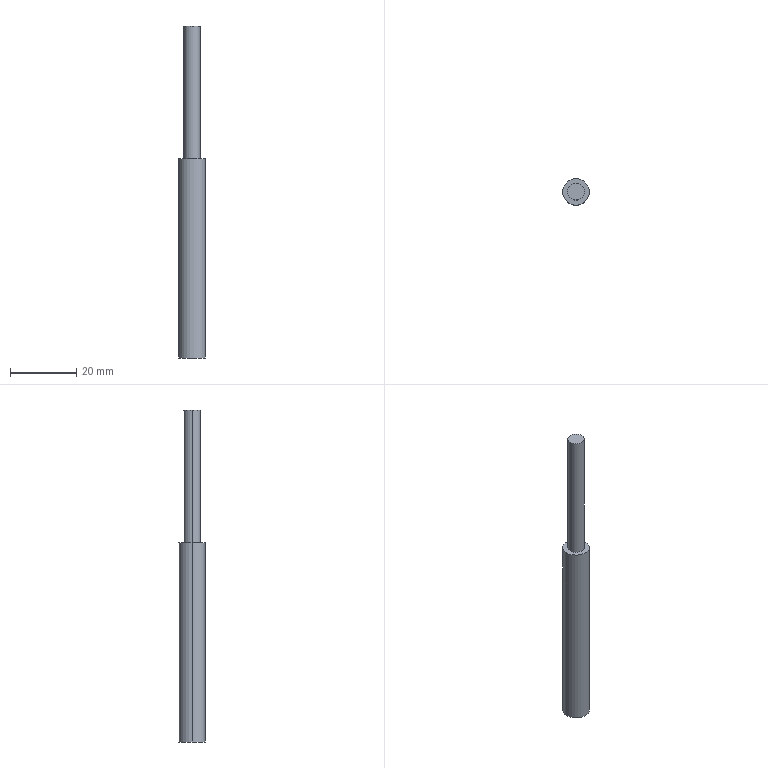Part | SolidWorks | features Extrusion 1, ICE 1 | 1 solid | 7 faces | box 8 x 8 x 100 mm | volume 3801 mm3 | cylinder 4 | plane 3 | commonest cylinder face diameters 5 x2 8 x2
STEP:
#1=CARTESIAN_POINT('',(2.5,0.,60.));
#2=VERTEX_POINT('',#1);
#3=CARTESIAN_POINT('',(-2.5,0.,60.));
#4=VERTEX_POINT('',#3);
#5=CARTESIAN_POINT('',(0.,0.,60.));
#6=DIRECTION('',(0.,0.,1.));
#7=DIRECTION('',(1.,0.,0.));
#8=AXIS2_PLACEMENT_3D('',#5,#6,#7);
#9=CIRCLE('',#8,2.5);
#10=EDGE_CURVE('',#2,#4,#9,.T.);
#11=ORIENTED_EDGE('',*,*,#10,.T.);
#12=CARTESIAN_POINT('',(-2.5,0.,100.));
#13=VERTEX_POINT('',#12);
#14=CARTESIAN_POINT('',(-2.5,0.,60.));
#15=DIRECTION('',(0.,0.,1.));
#16=VECTOR('',#15,1000.);
#17=LINE('',#14,#16);
#18=EDGE_CURVE('',#4,#13,#17,.T.);
#19=ORIENTED_EDGE('',*,*,#18,.T.);
#20=CARTESIAN_POINT('',(2.5,0.,100.));
#21=VERTEX_POINT('',#20);
#22=CARTESIAN_POINT('',(0.,0.,100.));
#23=DIRECTION('',(0.,0.,1.));
#24=DIRECTION('',(1.,0.,0.));
#25=AXIS2_PLACEMENT_3D('',#22,#23,#24);
#26=CIRCLE('',#25,2.5);
#27=EDGE_CURVE('',#21,#13,#26,.T.);
#28=ORIENTED_EDGE('',*,*,#27,.F.);
#29=CARTESIAN_POINT('',(2.5,0.,60.));
#30=DIRECTION('',(0.,0.,1.));
#31=VECTOR('',#30,1000.);
#32=LINE('',#29,#31);
#33=EDGE_CURVE('',#2,#21,#32,.T.);
#34=ORIENTED_EDGE('',*,*,#33,.F.);
#35=EDGE_LOOP('',(#11,#19,#28,#34));
#36=FACE_OUTER_BOUND('',#35,.T.);
#37=CARTESIAN_POINT('',(0.,0.,60.));
#38=DIRECTION('',(0.,0.,1.));
#39=DIRECTION('',(1.,0.,0.));
#40=AXIS2_PLACEMENT_3D('',#37,#38,#39);
#41=CYLINDRICAL_SURFACE('',#40,2.5);
#42=ADVANCED_FACE('',(#36),#41,.T.);
#43=CARTESIAN_POINT('',(4.,0.,60.));
#44=VERTEX_POINT('',#43);
#45=CARTESIAN_POINT('',(-4.,0.,60.));
#46=VERTEX_POINT('',#45);
#47=CARTESIAN_POINT('',(0.,0.,60.));
#48=DIRECTION('',(0.,0.,1.));
#49=DIRECTION('',(1.,0.,0.));
#50=AXIS2_PLACEMENT_3D('',#47,#48,#49);
#51=CIRCLE('',#50,4.);
#52=EDGE_CURVE('',#44,#46,#51,.T.);
#53=ORIENTED_EDGE('',*,*,#52,.F.);
#54=CARTESIAN_POINT('',(4.,0.,0.));
#55=VERTEX_POINT('',#54);
#56=CARTESIAN_POINT('',(4.,0.,100.));
#57=DIRECTION('',(0.,0.,-1.));
#58=VECTOR('',#57,1000.);
#59=LINE('',#56,#58);
#60=EDGE_CURVE('',#44,#55,#59,.T.);
#61=ORIENTED_EDGE('',*,*,#60,.T.);
#62=CARTESIAN_POINT('',(-4.,0.,0.));
#63=VERTEX_POINT('',#62);
#64=CARTESIAN_POINT('',(0.,0.,0.));
#65=DIRECTION('',(0.,0.,1.));
#66=DIRECTION('',(1.,0.,0.));
#67=AXIS2_PLACEMENT_3D('',#64,#65,#66);
#68=CIRCLE('',#67,4.);
#69=EDGE_CURVE('',#55,#63,#68,.T.);
#70=ORIENTED_EDGE('',*,*,#69,.T.);
#71=CARTESIAN_POINT('',(-4.,0.,100.));
#72=DIRECTION('',(0.,0.,-1.));
#73=VECTOR('',#72,1000.);
#74=LINE('',#71,#73);
#75=EDGE_CURVE('',#46,#63,#74,.T.);
#76=ORIENTED_EDGE('',*,*,#75,.F.);
#77=EDGE_LOOP('',(#53,#61,#70,#76));
#78=FACE_OUTER_BOUND('',#77,.T.);
#79=CARTESIAN_POINT('',(0.,0.,100.));
#80=DIRECTION('',(0.,0.,-1.));
#81=DIRECTION('',(-1.,0.,0.));
#82=AXIS2_PLACEMENT_3D('',#79,#80,#81);
#83=CYLINDRICAL_SURFACE('',#82,4.);
#84=ADVANCED_FACE('',(#78),#83,.T.);
#85=ORIENTED_EDGE('',*,*,#60,.F.);
#86=CARTESIAN_POINT('',(0.,0.,60.));
#87=DIRECTION('',(0.,0.,1.));
#88=DIRECTION('',(1.,0.,0.));
#89=AXIS2_PLACEMENT_3D('',#86,#87,#88);
#90=CIRCLE('',#89,4.);
#91=EDGE_CURVE('',#46,#44,#90,.T.);
#92=ORIENTED_EDGE('',*,*,#91,.F.);
#93=ORIENTED_EDGE('',*,*,#75,.T.);
#94=CARTESIAN_POINT('',(0.,0.,0.));
#95=DIRECTION('',(0.,0.,1.));
#96=DIRECTION('',(1.,0.,0.));
#97=AXIS2_PLACEMENT_3D('',#94,#95,#96);
#98=CIRCLE('',#97,4.);
#99=EDGE_CURVE('',#63,#55,#98,.T.);
#100=ORIENTED_EDGE('',*,*,#99,.T.);
#101=EDGE_LOOP('',(#85,#92,#93,#100));
#102=FACE_OUTER_BOUND('',#101,.T.);
#103=CARTESIAN_POINT('',(0.,0.,100.));
#104=DIRECTION('',(0.,0.,-1.));
#105=DIRECTION('',(-1.,0.,0.));
#106=AXIS2_PLACEMENT_3D('',#103,#104,#105);
#107=CYLINDRICAL_SURFACE('',#106,4.);
#108=ADVANCED_FACE('',(#102),#107,.T.);
#109=ORIENTED_EDGE('',*,*,#99,.F.);
#110=ORIENTED_EDGE('',*,*,#69,.F.);
#111=EDGE_LOOP('',(#109,#110));
#112=FACE_OUTER_BOUND('',#111,.T.);
#113=CARTESIAN_POINT('',(0.,0.,0.));
#114=DIRECTION('',(0.,0.,1.));
#115=DIRECTION('',(1.,0.,0.));
#116=AXIS2_PLACEMENT_3D('',#113,#114,#115);
#117=PLANE('',#116);
#118=ADVANCED_FACE('',(#112),#117,.F.);
#119=ORIENTED_EDGE('',*,*,#10,.F.);
#120=CARTESIAN_POINT('',(0.,0.,60.));
#121=DIRECTION('',(0.,0.,1.));
#122=DIRECTION('',(1.,0.,0.));
#123=AXIS2_PLACEMENT_3D('',#120,#121,#122);
#124=CIRCLE('',#123,2.5);
#125=EDGE_CURVE('',#4,#2,#124,.T.);
#126=ORIENTED_EDGE('',*,*,#125,.F.);
#127=EDGE_LOOP('',(#119,#126));
#128=FACE_BOUND('',#127,.T.);
#129=ORIENTED_EDGE('',*,*,#91,.T.);
#130=ORIENTED_EDGE('',*,*,#52,.T.);
#131=EDGE_LOOP('',(#129,#130));
#132=FACE_OUTER_BOUND('',#131,.T.);
#133=CARTESIAN_POINT('',(0.,0.,60.));
#134=DIRECTION('',(0.,0.,1.));
#135=DIRECTION('',(1.,0.,0.));
#136=AXIS2_PLACEMENT_3D('',#133,#134,#135);
#137=PLANE('',#136);
#138=ADVANCED_FACE('',(#128,#132),#137,.T.);
#139=ORIENTED_EDGE('',*,*,#18,.F.);
#140=ORIENTED_EDGE('',*,*,#125,.T.);
#141=ORIENTED_EDGE('',*,*,#33,.T.);
#142=CARTESIAN_POINT('',(0.,0.,100.));
#143=DIRECTION('',(0.,0.,1.));
#144=DIRECTION('',(1.,0.,0.));
#145=AXIS2_PLACEMENT_3D('',#142,#143,#144);
#146=CIRCLE('',#145,2.5);
#147=EDGE_CURVE('',#13,#21,#146,.T.);
#148=ORIENTED_EDGE('',*,*,#147,.F.);
#149=EDGE_LOOP('',(#139,#140,#141,#148));
#150=FACE_OUTER_BOUND('',#149,.T.);
#151=CARTESIAN_POINT('',(0.,0.,60.));
#152=DIRECTION('',(0.,0.,1.));
#153=DIRECTION('',(1.,0.,0.));
#154=AXIS2_PLACEMENT_3D('',#151,#152,#153);
#155=CYLINDRICAL_SURFACE('',#154,2.5);
#156=ADVANCED_FACE('',(#150),#155,.T.);
#157=ORIENTED_EDGE('',*,*,#27,.T.);
#158=ORIENTED_EDGE('',*,*,#147,.T.);
#159=EDGE_LOOP('',(#157,#158));
#160=FACE_OUTER_BOUND('',#159,.T.);
#161=CARTESIAN_POINT('',(0.,0.,100.));
#162=DIRECTION('',(0.,0.,1.));
#163=DIRECTION('',(1.,0.,0.));
#164=AXIS2_PLACEMENT_3D('',#161,#162,#163);
#165=PLANE('',#164);
#166=ADVANCED_FACE('',(#160),#165,.T.);
#167=CLOSED_SHELL('',(#42,#84,#108,#118,#138,#156,#166));
#168=MANIFOLD_SOLID_BREP('',#167);
#169=CARTESIAN_POINT('',(0.,0.,0.));
#170=DIRECTION('',(0.,0.,1.));
#171=DIRECTION('',(1.,0.,0.));
#172=AXIS2_PLACEMENT_3D('',#169,#170,#171);
#173=(LENGTH_UNIT()NAMED_UNIT(*)SI_UNIT(.MILLI.,.METRE.));
#174=UNCERTAINTY_MEASURE_WITH_UNIT(LENGTH_MEASURE(0.00001),#173,'','');
#175=(NAMED_UNIT(*)PLANE_ANGLE_UNIT()SI_UNIT($,.RADIAN.));
#176=(NAMED_UNIT(*)SI_UNIT($,.STERADIAN.)SOLID_ANGLE_UNIT());
#177=(GEOMETRIC_REPRESENTATION_CONTEXT(3)GLOBAL_UNCERTAINTY_ASSIGNED_CONTEXT((#174))GLOBAL_UNIT_ASSIGNED_CONTEXT((#173,#175,#176))REPRESENTATION_CONTEXT('',''));
#178=ADVANCED_BREP_SHAPE_REPRESENTATION('',(#168,#172),#177);